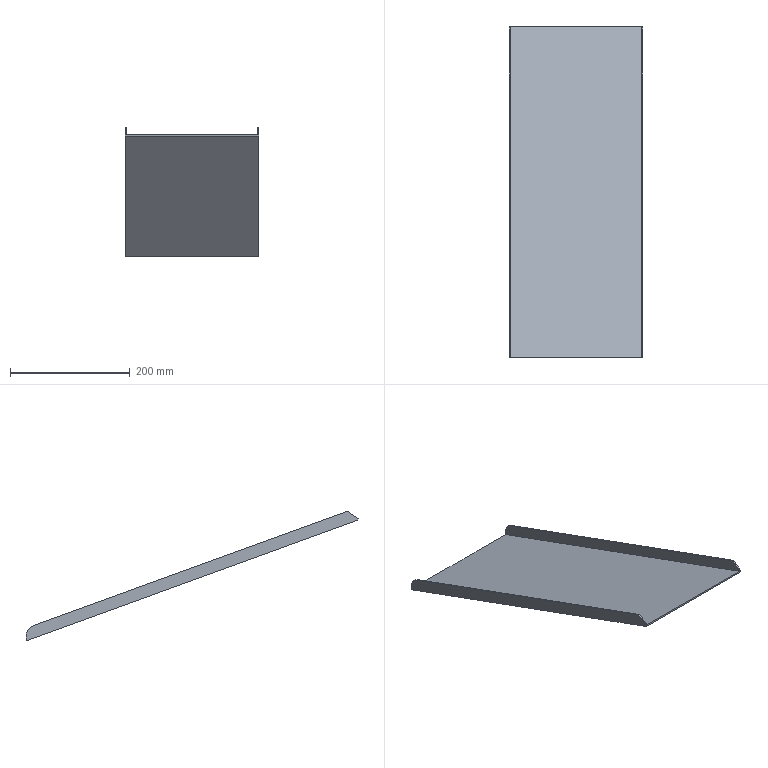Part | NX | features solid 2 | 1 solid | 14 faces | box 224.044 x 555.861 x 216.896 mm | volume 306885 mm3 | plane 9 | spline 3 | cylinder 2 | commonest cylinder face diameters 40 x2
STEP:
#1=CARTESIAN_POINT('',(-392.044,820.,-511.765));
#2=VERTEX_POINT('',#1);
#3=CARTESIAN_POINT('',(-172.,820.,-511.765));
#4=VERTEX_POINT('',#3);
#5=CARTESIAN_POINT('',(-394.044,820.,-511.765));
#6=DIRECTION('',(-1.,0.,0.));
#7=VECTOR('',#6,1000.);
#8=LINE('',#5,#7);
#9=EDGE_CURVE('',#2,#4,#8,.F.);
#10=ORIENTED_EDGE('',*,*,#9,.F.);
#11=CARTESIAN_POINT('',(-392.044,820.,-509.637));
#12=VERTEX_POINT('',#11);
#13=CARTESIAN_POINT('',(-392.044,820.,-700.));
#14=DIRECTION('',(0.,0.,-1.));
#15=VECTOR('',#14,1000.);
#16=LINE('',#13,#15);
#17=EDGE_CURVE('',#2,#12,#16,.F.);
#18=ORIENTED_EDGE('',*,*,#17,.T.);
#19=CARTESIAN_POINT('',(-172.,820.,-509.637));
#20=VERTEX_POINT('',#19);
#21=CARTESIAN_POINT('',(675.,820.,-509.637));
#22=DIRECTION('',(1.,0.,0.));
#23=VECTOR('',#22,1000.);
#24=LINE('',#21,#23);
#25=EDGE_CURVE('',#20,#12,#24,.F.);
#26=ORIENTED_EDGE('',*,*,#25,.F.);
#27=CARTESIAN_POINT('',(-172.,820.,-700.));
#28=DIRECTION('',(0.,0.,-1.));
#29=VECTOR('',#28,1000.);
#30=LINE('',#27,#29);
#31=EDGE_CURVE('',#4,#20,#30,.F.);
#32=ORIENTED_EDGE('',*,*,#31,.F.);
#33=EDGE_LOOP('',(#10,#18,#26,#32));
#34=FACE_BOUND('',#33,.T.);
#35=CARTESIAN_POINT('',(675.,820.,-700.));
#36=DIRECTION('',(0.,-1.,0.));
#37=DIRECTION('',(-1.,0.,0.));
#38=AXIS2_PLACEMENT_3D('',#35,#36,#37);
#39=PLANE('',#38);
#40=ADVANCED_FACE('',(#34),#39,.F.);
#41=CARTESIAN_POINT('',(-392.044,265.649,-307.869));
#42=VERTEX_POINT('',#41);
#43=CARTESIAN_POINT('',(-392.044,1206.032,-650.141));
#44=DIRECTION('',(0.,0.9397,-0.342));
#45=VECTOR('',#44,1000.);
#46=LINE('',#43,#45);
#47=EDGE_CURVE('',#42,#12,#46,.T.);
#48=ORIENTED_EDGE('',*,*,#47,.F.);
#49=CARTESIAN_POINT('',(-172.,265.645,-307.868));
#50=VERTEX_POINT('',#49);
#51=CARTESIAN_POINT('',(-392.044,265.649,-307.869));
#52=CARTESIAN_POINT('',(-382.876,265.644,-307.868));
#53=CARTESIAN_POINT('',(-364.539,265.649,-307.869));
#54=CARTESIAN_POINT('',(-341.617,265.581,-307.845));
#55=CARTESIAN_POINT('',(-323.28,265.66,-307.873));
#56=CARTESIAN_POINT('',(-309.528,265.272,-307.732));
#57=CARTESIAN_POINT('',(-295.775,265.417,-307.785));
#58=CARTESIAN_POINT('',(-277.438,265.558,-307.836));
#59=CARTESIAN_POINT('',(-254.517,265.652,-307.871));
#60=CARTESIAN_POINT('',(-217.843,265.608,-307.855));
#61=CARTESIAN_POINT('',(-190.337,265.641,-307.866));
#62=CARTESIAN_POINT('',(-172.,265.645,-307.868));
#63=B_SPLINE_CURVE_WITH_KNOTS('',3,(#51,#52,#53,#54,#55,#56,#57,#58,#59,#60,#61,#62),.UNSPECIFIED.,.F.,.F.,(4,1,1,1,1,1,1,1,1,4),(0.,0.02751,0.05501,0.06876,0.08252,0.09627,0.11,0.1375,0.165,0.22),.UNSPECIFIED.);
#64=EDGE_CURVE('',#42,#50,#63,.T.);
#65=ORIENTED_EDGE('',*,*,#64,.T.);
#66=CARTESIAN_POINT('',(-172.,1206.032,-650.141));
#67=DIRECTION('',(0.,0.9397,-0.342));
#68=VECTOR('',#67,1000.);
#69=LINE('',#66,#68);
#70=EDGE_CURVE('',#50,#20,#69,.T.);
#71=ORIENTED_EDGE('',*,*,#70,.T.);
#72=ORIENTED_EDGE('',*,*,#25,.T.);
#73=EDGE_LOOP('',(#48,#65,#71,#72));
#74=FACE_BOUND('',#73,.T.);
#75=CARTESIAN_POINT('',(-394.044,1206.032,-650.141));
#76=DIRECTION('',(0.,-0.342,-0.9397));
#77=DIRECTION('',(-1.,0.,0.));
#78=AXIS2_PLACEMENT_3D('',#75,#76,#77);
#79=PLANE('',#78);
#80=ADVANCED_FACE('',(#74),#79,.F.);
#81=CARTESIAN_POINT('',(-170.,808.047,-486.131));
#82=VERTEX_POINT('',#81);
#83=CARTESIAN_POINT('',(-170.,282.56,-294.869));
#84=VERTEX_POINT('',#83);
#85=CARTESIAN_POINT('',(-170.,826.84,-492.971));
#86=DIRECTION('',(0.,-0.9397,0.342));
#87=VECTOR('',#86,1000.);
#88=LINE('',#85,#87);
#89=EDGE_CURVE('',#82,#84,#88,.T.);
#90=ORIENTED_EDGE('',*,*,#89,.T.);
#91=CARTESIAN_POINT('',(-170.,265.646,-306.713));
#92=VERTEX_POINT('',#91);
#93=CARTESIAN_POINT('',(-170.,282.56,-294.869));
#94=CARTESIAN_POINT('',(-170.,276.922,-298.817));
#95=CARTESIAN_POINT('',(-170.,271.284,-302.765));
#96=CARTESIAN_POINT('',(-170.,265.646,-306.713));
#97=B_SPLINE_CURVE_WITH_KNOTS('',3,(#93,#94,#95,#96),.UNSPECIFIED.,.F.,.F.,(4,4),(0.,1.),.UNSPECIFIED.);
#98=EDGE_CURVE('',#84,#92,#97,.T.);
#99=ORIENTED_EDGE('',*,*,#98,.T.);
#100=CARTESIAN_POINT('',(-170.,265.646,-309.996));
#101=VERTEX_POINT('',#100);
#102=CARTESIAN_POINT('',(-170.,265.646,-420.));
#103=DIRECTION('',(0.,0.,-1.));
#104=VECTOR('',#103,1000.);
#105=LINE('',#102,#104);
#106=EDGE_CURVE('',#101,#92,#105,.F.);
#107=ORIENTED_EDGE('',*,*,#106,.F.);
#108=CARTESIAN_POINT('',(-170.,820.,-511.765));
#109=VERTEX_POINT('',#108);
#110=CARTESIAN_POINT('',(-170.,1205.348,-652.02));
#111=DIRECTION('',(0.,-0.9397,0.342));
#112=VECTOR('',#111,1000.);
#113=LINE('',#110,#112);
#114=EDGE_CURVE('',#109,#101,#113,.T.);
#115=ORIENTED_EDGE('',*,*,#114,.F.);
#116=CARTESIAN_POINT('',(-170.,801.206,-504.925));
#117=DIRECTION('',(-1.,0.,0.));
#118=DIRECTION('',(0.,0.,1.));
#119=AXIS2_PLACEMENT_3D('',#116,#117,#118);
#120=CIRCLE('',#119,20.);
#121=EDGE_CURVE('',#109,#82,#120,.F.);
#122=ORIENTED_EDGE('',*,*,#121,.T.);
#123=EDGE_LOOP('',(#90,#99,#107,#115,#122));
#124=FACE_BOUND('',#123,.T.);
#125=CARTESIAN_POINT('',(-170.,1206.032,-650.141));
#126=DIRECTION('',(1.,0.,0.));
#127=DIRECTION('',(0.,0.,-1.));
#128=AXIS2_PLACEMENT_3D('',#125,#126,#127);
#129=PLANE('',#128);
#130=ADVANCED_FACE('',(#124),#129,.T.);
#131=CARTESIAN_POINT('',(-394.044,265.65,-309.998));
#132=VERTEX_POINT('',#131);
#133=CARTESIAN_POINT('',(-394.044,265.65,-306.715));
#134=VERTEX_POINT('',#133);
#135=CARTESIAN_POINT('',(-394.044,265.65,-308.356));
#136=DIRECTION('',(0.,0.,-1.));
#137=VECTOR('',#136,1000.);
#138=LINE('',#135,#137);
#139=EDGE_CURVE('',#132,#134,#138,.F.);
#140=ORIENTED_EDGE('',*,*,#139,.T.);
#141=CARTESIAN_POINT('',(-394.044,282.564,-294.871));
#142=VERTEX_POINT('',#141);
#143=CARTESIAN_POINT('',(-394.044,265.65,-306.715));
#144=CARTESIAN_POINT('',(-394.044,271.288,-302.767));
#145=CARTESIAN_POINT('',(-394.044,276.926,-298.819));
#146=CARTESIAN_POINT('',(-394.044,282.564,-294.871));
#147=B_SPLINE_CURVE_WITH_KNOTS('',3,(#143,#144,#145,#146),.UNSPECIFIED.,.F.,.F.,(4,4),(0.,0.02065),.UNSPECIFIED.);
#148=EDGE_CURVE('',#134,#142,#147,.T.);
#149=ORIENTED_EDGE('',*,*,#148,.T.);
#150=CARTESIAN_POINT('',(-394.044,808.047,-486.131));
#151=VERTEX_POINT('',#150);
#152=CARTESIAN_POINT('',(-394.044,1212.188,-633.226));
#153=DIRECTION('',(0.,-0.9397,0.342));
#154=VECTOR('',#153,1000.);
#155=LINE('',#152,#154);
#156=EDGE_CURVE('',#151,#142,#155,.T.);
#157=ORIENTED_EDGE('',*,*,#156,.F.);
#158=CARTESIAN_POINT('',(-394.044,820.,-511.765));
#159=VERTEX_POINT('',#158);
#160=CARTESIAN_POINT('',(-394.044,801.206,-504.925));
#161=DIRECTION('',(-1.,0.,0.));
#162=DIRECTION('',(0.,0.,1.));
#163=AXIS2_PLACEMENT_3D('',#160,#161,#162);
#164=CIRCLE('',#163,20.);
#165=EDGE_CURVE('',#151,#159,#164,.T.);
#166=ORIENTED_EDGE('',*,*,#165,.T.);
#167=CARTESIAN_POINT('',(-394.044,1205.348,-652.02));
#168=DIRECTION('',(0.,0.9397,-0.342));
#169=VECTOR('',#168,1000.);
#170=LINE('',#167,#169);
#171=EDGE_CURVE('',#159,#132,#170,.F.);
#172=ORIENTED_EDGE('',*,*,#171,.T.);
#173=EDGE_LOOP('',(#140,#149,#157,#166,#172));
#174=FACE_BOUND('',#173,.T.);
#175=CARTESIAN_POINT('',(-394.044,1205.348,-652.02));
#176=DIRECTION('',(-1.,0.,0.));
#177=DIRECTION('',(0.,0.,1.));
#178=AXIS2_PLACEMENT_3D('',#175,#176,#177);
#179=PLANE('',#178);
#180=ADVANCED_FACE('',(#174),#179,.T.);
#181=CARTESIAN_POINT('',(-394.044,265.65,-309.998));
#182=CARTESIAN_POINT('',(-384.709,265.645,-309.996));
#183=CARTESIAN_POINT('',(-366.039,265.65,-309.998));
#184=CARTESIAN_POINT('',(-342.701,265.58,-309.973));
#185=CARTESIAN_POINT('',(-324.03,265.664,-310.003));
#186=CARTESIAN_POINT('',(-310.028,265.279,-309.863));
#187=CARTESIAN_POINT('',(-296.025,265.412,-309.911));
#188=CARTESIAN_POINT('',(-277.355,265.56,-309.966));
#189=CARTESIAN_POINT('',(-254.017,265.651,-309.999));
#190=CARTESIAN_POINT('',(-216.676,265.609,-309.983));
#191=CARTESIAN_POINT('',(-188.67,265.641,-309.995));
#192=CARTESIAN_POINT('',(-170.,265.646,-309.996));
#193=B_SPLINE_CURVE_WITH_KNOTS('',3,(#181,#182,#183,#184,#185,#186,#187,#188,#189,#190,#191,#192),.UNSPECIFIED.,.F.,.F.,(4,1,1,1,1,1,1,1,1,4),(0.003,0.03101,0.05901,0.07301,0.08702,0.101,0.115,0.143,0.171,0.227),.UNSPECIFIED.);
#194=EDGE_CURVE('',#132,#101,#193,.T.);
#195=ORIENTED_EDGE('',*,*,#194,.F.);
#196=ORIENTED_EDGE('',*,*,#171,.F.);
#197=CARTESIAN_POINT('',(-394.044,820.,-511.765));
#198=DIRECTION('',(-1.,0.,0.));
#199=VECTOR('',#198,1000.);
#200=LINE('',#197,#199);
#201=EDGE_CURVE('',#159,#2,#200,.F.);
#202=ORIENTED_EDGE('',*,*,#201,.T.);
#203=ORIENTED_EDGE('',*,*,#9,.T.);
#204=CARTESIAN_POINT('',(-170.,820.,-511.765));
#205=DIRECTION('',(1.,0.,0.));
#206=VECTOR('',#205,1000.);
#207=LINE('',#204,#206);
#208=EDGE_CURVE('',#109,#4,#207,.F.);
#209=ORIENTED_EDGE('',*,*,#208,.F.);
#210=ORIENTED_EDGE('',*,*,#114,.T.);
#211=EDGE_LOOP('',(#195,#196,#202,#203,#209,#210));
#212=FACE_BOUND('',#211,.T.);
#213=CARTESIAN_POINT('',(-394.044,1205.348,-652.02));
#214=DIRECTION('',(0.,-0.342,-0.9397));
#215=DIRECTION('',(-1.,0.,0.));
#216=AXIS2_PLACEMENT_3D('',#213,#214,#215);
#217=PLANE('',#216);
#218=ADVANCED_FACE('',(#212),#217,.T.);
#219=CARTESIAN_POINT('',(-172.,808.047,-486.131));
#220=VERTEX_POINT('',#219);
#221=CARTESIAN_POINT('',(-172.,282.56,-294.869));
#222=VERTEX_POINT('',#221);
#223=CARTESIAN_POINT('',(-172.,826.84,-492.971));
#224=DIRECTION('',(0.,-0.9397,0.342));
#225=VECTOR('',#224,1000.);
#226=LINE('',#223,#225);
#227=EDGE_CURVE('',#220,#222,#226,.T.);
#228=ORIENTED_EDGE('',*,*,#227,.T.);
#229=CARTESIAN_POINT('',(-172.,282.56,-294.869));
#230=CARTESIAN_POINT('',(-171.333,282.56,-294.869));
#231=CARTESIAN_POINT('',(-170.667,282.56,-294.869));
#232=CARTESIAN_POINT('',(-170.,282.56,-294.869));
#233=B_SPLINE_CURVE_WITH_KNOTS('',3,(#229,#230,#231,#232),.UNSPECIFIED.,.F.,.F.,(4,4),(0.,1.),.UNSPECIFIED.);
#234=EDGE_CURVE('',#222,#84,#233,.T.);
#235=ORIENTED_EDGE('',*,*,#234,.T.);
#236=ORIENTED_EDGE('',*,*,#89,.F.);
#237=CARTESIAN_POINT('',(-170.,808.047,-486.131));
#238=DIRECTION('',(-1.,0.,0.));
#239=VECTOR('',#238,1000.);
#240=LINE('',#237,#239);
#241=EDGE_CURVE('',#82,#220,#240,.T.);
#242=ORIENTED_EDGE('',*,*,#241,.T.);
#243=EDGE_LOOP('',(#228,#235,#236,#242));
#244=FACE_BOUND('',#243,.T.);
#245=CARTESIAN_POINT('',(-170.,826.84,-492.971));
#246=DIRECTION('',(0.,-0.342,-0.9397));
#247=DIRECTION('',(0.,-0.9397,0.342));
#248=AXIS2_PLACEMENT_3D('',#245,#246,#247);
#249=PLANE('',#248);
#250=ADVANCED_FACE('',(#244),#249,.F.);
#251=CARTESIAN_POINT('',(-172.,265.645,-306.713));
#252=VERTEX_POINT('',#251);
#253=CARTESIAN_POINT('',(-172.,265.645,-420.));
#254=DIRECTION('',(0.,0.,-1.));
#255=VECTOR('',#254,1000.);
#256=LINE('',#253,#255);
#257=EDGE_CURVE('',#252,#50,#256,.T.);
#258=ORIENTED_EDGE('',*,*,#257,.F.);
#259=CARTESIAN_POINT('',(-172.,265.645,-306.713));
#260=CARTESIAN_POINT('',(-172.,271.283,-302.765));
#261=CARTESIAN_POINT('',(-172.,276.921,-298.817));
#262=CARTESIAN_POINT('',(-172.,282.56,-294.869));
#263=B_SPLINE_CURVE_WITH_KNOTS('',3,(#259,#260,#261,#262),.UNSPECIFIED.,.F.,.F.,(4,4),(0.,1.),.UNSPECIFIED.);
#264=EDGE_CURVE('',#252,#222,#263,.T.);
#265=ORIENTED_EDGE('',*,*,#264,.T.);
#266=ORIENTED_EDGE('',*,*,#227,.F.);
#267=CARTESIAN_POINT('',(-172.,801.206,-504.925));
#268=DIRECTION('',(-1.,0.,0.));
#269=DIRECTION('',(0.,0.,1.));
#270=AXIS2_PLACEMENT_3D('',#267,#268,#269);
#271=CIRCLE('',#270,20.);
#272=EDGE_CURVE('',#220,#4,#271,.T.);
#273=ORIENTED_EDGE('',*,*,#272,.T.);
#274=ORIENTED_EDGE('',*,*,#31,.T.);
#275=ORIENTED_EDGE('',*,*,#70,.F.);
#276=EDGE_LOOP('',(#258,#265,#266,#273,#274,#275));
#277=FACE_BOUND('',#276,.T.);
#278=CARTESIAN_POINT('',(-172.,820.,-511.765));
#279=DIRECTION('',(-1.,0.,0.));
#280=DIRECTION('',(0.,0.,1.));
#281=AXIS2_PLACEMENT_3D('',#278,#279,#280);
#282=PLANE('',#281);
#283=ADVANCED_FACE('',(#277),#282,.T.);
#284=ORIENTED_EDGE('',*,*,#121,.F.);
#285=ORIENTED_EDGE('',*,*,#208,.T.);
#286=ORIENTED_EDGE('',*,*,#272,.F.);
#287=ORIENTED_EDGE('',*,*,#241,.F.);
#288=EDGE_LOOP('',(#284,#285,#286,#287));
#289=FACE_BOUND('',#288,.T.);
#290=CARTESIAN_POINT('',(-170.,801.206,-504.925));
#291=DIRECTION('',(-1.,0.,0.));
#292=DIRECTION('',(0.,0.,1.));
#293=AXIS2_PLACEMENT_3D('',#290,#291,#292);
#294=CYLINDRICAL_SURFACE('',#293,20.);
#295=ADVANCED_FACE('',(#289),#294,.T.);
#296=ORIENTED_EDGE('',*,*,#156,.T.);
#297=CARTESIAN_POINT('',(-392.044,282.563,-294.87));
#298=VERTEX_POINT('',#297);
#299=CARTESIAN_POINT('',(-394.044,282.564,-294.871));
#300=CARTESIAN_POINT('',(-393.378,282.564,-294.871));
#301=CARTESIAN_POINT('',(-392.711,282.564,-294.871));
#302=CARTESIAN_POINT('',(-392.044,282.563,-294.87));
#303=B_SPLINE_CURVE_WITH_KNOTS('',3,(#299,#300,#301,#302),.UNSPECIFIED.,.F.,.F.,(4,4),(0.6,1.),.UNSPECIFIED.);
#304=EDGE_CURVE('',#142,#298,#303,.T.);
#305=ORIENTED_EDGE('',*,*,#304,.T.);
#306=CARTESIAN_POINT('',(-392.044,808.047,-486.131));
#307=VERTEX_POINT('',#306);
#308=CARTESIAN_POINT('',(-392.044,826.84,-492.971));
#309=DIRECTION('',(0.,0.9397,-0.342));
#310=VECTOR('',#309,1000.);
#311=LINE('',#308,#310);
#312=EDGE_CURVE('',#307,#298,#311,.F.);
#313=ORIENTED_EDGE('',*,*,#312,.F.);
#314=CARTESIAN_POINT('',(-399.044,808.047,-486.131));
#315=DIRECTION('',(-1.,0.,0.));
#316=VECTOR('',#315,1000.);
#317=LINE('',#314,#316);
#318=EDGE_CURVE('',#307,#151,#317,.T.);
#319=ORIENTED_EDGE('',*,*,#318,.T.);
#320=EDGE_LOOP('',(#296,#305,#313,#319));
#321=FACE_BOUND('',#320,.T.);
#322=CARTESIAN_POINT('',(-399.044,826.84,-492.971));
#323=DIRECTION('',(0.,-0.342,-0.9397));
#324=DIRECTION('',(0.,-0.9397,0.342));
#325=AXIS2_PLACEMENT_3D('',#322,#323,#324);
#326=PLANE('',#325);
#327=ADVANCED_FACE('',(#321),#326,.F.);
#328=ORIENTED_EDGE('',*,*,#312,.T.);
#329=CARTESIAN_POINT('',(-392.044,265.649,-306.714));
#330=VERTEX_POINT('',#329);
#331=CARTESIAN_POINT('',(-392.044,282.563,-294.87));
#332=CARTESIAN_POINT('',(-392.044,276.925,-298.818));
#333=CARTESIAN_POINT('',(-392.044,271.287,-302.766));
#334=CARTESIAN_POINT('',(-392.044,265.649,-306.714));
#335=B_SPLINE_CURVE_WITH_KNOTS('',3,(#331,#332,#333,#334),.UNSPECIFIED.,.F.,.F.,(4,4),(0.,1.),.UNSPECIFIED.);
#336=EDGE_CURVE('',#298,#330,#335,.T.);
#337=ORIENTED_EDGE('',*,*,#336,.T.);
#338=CARTESIAN_POINT('',(-392.044,265.649,-420.));
#339=DIRECTION('',(0.,0.,-1.));
#340=VECTOR('',#339,1000.);
#341=LINE('',#338,#340);
#342=EDGE_CURVE('',#330,#42,#341,.T.);
#343=ORIENTED_EDGE('',*,*,#342,.T.);
#344=ORIENTED_EDGE('',*,*,#47,.T.);
#345=ORIENTED_EDGE('',*,*,#17,.F.);
#346=CARTESIAN_POINT('',(-392.044,801.206,-504.925));
#347=DIRECTION('',(-1.,0.,0.));
#348=DIRECTION('',(0.,0.,1.));
#349=AXIS2_PLACEMENT_3D('',#346,#347,#348);
#350=CIRCLE('',#349,20.);
#351=EDGE_CURVE('',#2,#307,#350,.F.);
#352=ORIENTED_EDGE('',*,*,#351,.T.);
#353=EDGE_LOOP('',(#328,#337,#343,#344,#345,#352));
#354=FACE_BOUND('',#353,.T.);
#355=CARTESIAN_POINT('',(-392.044,1205.348,-652.02));
#356=DIRECTION('',(-1.,0.,0.));
#357=DIRECTION('',(0.,0.,1.));
#358=AXIS2_PLACEMENT_3D('',#355,#356,#357);
#359=PLANE('',#358);
#360=ADVANCED_FACE('',(#354),#359,.F.);
#361=ORIENTED_EDGE('',*,*,#165,.F.);
#362=ORIENTED_EDGE('',*,*,#318,.F.);
#363=ORIENTED_EDGE('',*,*,#351,.F.);
#364=ORIENTED_EDGE('',*,*,#201,.F.);
#365=EDGE_LOOP('',(#361,#362,#363,#364));
#366=FACE_BOUND('',#365,.T.);
#367=CARTESIAN_POINT('',(-399.044,801.206,-504.925));
#368=DIRECTION('',(1.,0.,0.));
#369=DIRECTION('',(0.,0.,-1.));
#370=AXIS2_PLACEMENT_3D('',#367,#368,#369);
#371=CYLINDRICAL_SURFACE('',#370,20.);
#372=ADVANCED_FACE('',(#366),#371,.T.);
#373=ORIENTED_EDGE('',*,*,#342,.F.);
#374=CARTESIAN_POINT('',(-392.044,265.649,-306.714));
#375=CARTESIAN_POINT('',(-392.711,265.649,-306.714));
#376=CARTESIAN_POINT('',(-393.378,265.65,-306.714));
#377=CARTESIAN_POINT('',(-394.044,265.65,-306.715));
#378=B_SPLINE_CURVE_WITH_KNOTS('',3,(#374,#375,#376,#377),.UNSPECIFIED.,.F.,.F.,(4,4),(0.,0.4),.UNSPECIFIED.);
#379=EDGE_CURVE('',#330,#134,#378,.T.);
#380=ORIENTED_EDGE('',*,*,#379,.T.);
#381=ORIENTED_EDGE('',*,*,#139,.F.);
#382=ORIENTED_EDGE('',*,*,#194,.T.);
#383=ORIENTED_EDGE('',*,*,#106,.T.);
#384=CARTESIAN_POINT('',(-170.,265.646,-306.713));
#385=CARTESIAN_POINT('',(-170.667,265.645,-306.713));
#386=CARTESIAN_POINT('',(-171.333,265.645,-306.713));
#387=CARTESIAN_POINT('',(-172.,265.645,-306.713));
#388=B_SPLINE_CURVE_WITH_KNOTS('',3,(#384,#385,#386,#387),.UNSPECIFIED.,.F.,.F.,(4,4),(0.,1.),.UNSPECIFIED.);
#389=EDGE_CURVE('',#92,#252,#388,.T.);
#390=ORIENTED_EDGE('',*,*,#389,.T.);
#391=ORIENTED_EDGE('',*,*,#257,.T.);
#392=ORIENTED_EDGE('',*,*,#64,.F.);
#393=EDGE_LOOP('',(#373,#380,#381,#382,#383,#390,#391,#392));
#394=FACE_BOUND('',#393,.T.);
#395=CARTESIAN_POINT('',(-394.044,265.65,-306.693));
#396=CARTESIAN_POINT('',(-394.044,265.65,-310.077));
#397=CARTESIAN_POINT('',(-384.044,265.645,-306.693));
#398=CARTESIAN_POINT('',(-384.044,265.645,-310.077));
#399=CARTESIAN_POINT('',(-374.043,265.639,-306.693));
#400=CARTESIAN_POINT('',(-374.043,265.639,-310.077));
#401=CARTESIAN_POINT('',(-364.042,265.634,-306.693));
#402=CARTESIAN_POINT('',(-364.042,265.634,-310.077));
#403=CARTESIAN_POINT('',(-363.233,265.633,-306.693));
#404=CARTESIAN_POINT('',(-363.233,265.633,-310.077));
#405=CARTESIAN_POINT('',(-355.475,265.629,-306.693));
#406=CARTESIAN_POINT('',(-355.475,265.629,-310.077));
#407=CARTESIAN_POINT('',(-344.102,265.622,-306.693));
#408=CARTESIAN_POINT('',(-344.102,265.622,-310.077));
#409=CARTESIAN_POINT('',(-331.712,265.604,-306.693));
#410=CARTESIAN_POINT('',(-331.712,265.604,-310.077));
#411=CARTESIAN_POINT('',(-324.733,265.598,-306.693));
#412=CARTESIAN_POINT('',(-324.733,265.598,-310.077));
#413=CARTESIAN_POINT('',(-320.466,265.567,-306.693));
#414=CARTESIAN_POINT('',(-320.466,265.567,-310.077));
#415=CARTESIAN_POINT('',(-316.238,265.475,-306.693));
#416=CARTESIAN_POINT('',(-316.238,265.475,-310.077));
#417=CARTESIAN_POINT('',(-311.164,265.363,-306.693));
#418=CARTESIAN_POINT('',(-311.164,265.363,-310.077));
#419=CARTESIAN_POINT('',(-305.076,265.333,-306.693));
#420=CARTESIAN_POINT('',(-305.076,265.333,-310.077));
#421=CARTESIAN_POINT('',(-297.793,265.396,-306.693));
#422=CARTESIAN_POINT('',(-297.793,265.396,-310.077));
#423=CARTESIAN_POINT('',(-289.399,265.458,-306.693));
#424=CARTESIAN_POINT('',(-289.399,265.458,-310.077));
#425=CARTESIAN_POINT('',(-278.989,265.541,-306.693));
#426=CARTESIAN_POINT('',(-278.989,265.541,-310.077));
#427=CARTESIAN_POINT('',(-268.929,265.619,-306.693));
#428=CARTESIAN_POINT('',(-268.929,265.619,-310.077));
#429=CARTESIAN_POINT('',(-258.644,265.632,-306.693));
#430=CARTESIAN_POINT('',(-258.644,265.632,-310.077));
#431=CARTESIAN_POINT('',(-248.025,265.624,-306.693));
#432=CARTESIAN_POINT('',(-248.025,265.624,-310.077));
#433=CARTESIAN_POINT('',(-226.868,265.624,-306.693));
#434=CARTESIAN_POINT('',(-226.868,265.624,-310.077));
#435=CARTESIAN_POINT('',(-200.897,265.637,-306.693));
#436=CARTESIAN_POINT('',(-200.897,265.637,-310.077));
#437=CARTESIAN_POINT('',(-178.423,265.644,-306.693));
#438=CARTESIAN_POINT('',(-178.423,265.644,-310.077));
#439=CARTESIAN_POINT('',(-170.,265.646,-306.693));
#440=CARTESIAN_POINT('',(-170.,265.646,-310.077));
#441=B_SPLINE_SURFACE_WITH_KNOTS('',3,1,((#395,#396),(#397,#398),(#399,#400),(#401,#402),(#403,#404),(#405,#406),(#407,#408),(#409,#410),(#411,#412),(#413,#414),(#415,#416),(#417,#418),(#419,#420),(#421,#422),(#423,#424),(#425,#426),(#427,#428),(#429,#430),(#431,#432),(#433,#434),(#435,#436),(#437,#438),(#439,#440)),.SURF_OF_LINEAR_EXTRUSION.,.F.,.F.,.F.,(4,3,1,1,1,1,1,1,1,1,1,1,1,1,1,1,1,1,4),(2,2),(0.2365,0.2855,0.2895,0.3235,0.3405,0.349,0.3575,0.366,0.3745,0.383,0.3915,0.4085,0.4255,0.4426,0.4596,0.4766,0.4936,0.5616,0.6024),(0.3868,0.3901),.UNSPECIFIED.);
#442=ADVANCED_FACE('',(#394),#441,.F.);
#443=ORIENTED_EDGE('',*,*,#264,.F.);
#444=ORIENTED_EDGE('',*,*,#389,.F.);
#445=ORIENTED_EDGE('',*,*,#98,.F.);
#446=ORIENTED_EDGE('',*,*,#234,.F.);
#447=EDGE_LOOP('',(#443,#444,#445,#446));
#448=FACE_BOUND('',#447,.T.);
#449=CARTESIAN_POINT('',(-172.015,282.56,-294.869));
#450=CARTESIAN_POINT('',(-171.339,282.56,-294.869));
#451=CARTESIAN_POINT('',(-170.664,282.56,-294.869));
#452=CARTESIAN_POINT('',(-169.988,282.56,-294.869));
#453=CARTESIAN_POINT('',(-172.012,265.645,-306.713));
#454=CARTESIAN_POINT('',(-171.336,265.645,-306.713));
#455=CARTESIAN_POINT('',(-170.661,265.645,-306.713));
#456=CARTESIAN_POINT('',(-169.985,265.646,-306.713));
#457=B_SPLINE_SURFACE_WITH_KNOTS('',1,3,((#449,#450,#451,#452),(#453,#454,#455,#456)),.RULED_SURF.,.F.,.F.,.F.,(2,2),(4,4),(0.,1.),(0.1835,0.1856),.PIECEWISE_BEZIER_KNOTS.);
#458=ADVANCED_FACE('',(#448),#457,.T.);
#459=ORIENTED_EDGE('',*,*,#336,.F.);
#460=ORIENTED_EDGE('',*,*,#304,.F.);
#461=ORIENTED_EDGE('',*,*,#148,.F.);
#462=ORIENTED_EDGE('',*,*,#379,.F.);
#463=EDGE_LOOP('',(#459,#460,#461,#462));
#464=FACE_BOUND('',#463,.T.);
#465=CARTESIAN_POINT('',(-392.032,265.649,-306.714));
#466=CARTESIAN_POINT('',(-392.709,265.649,-306.714));
#467=CARTESIAN_POINT('',(-393.386,265.65,-306.714));
#468=CARTESIAN_POINT('',(-394.063,265.65,-306.715));
#469=CARTESIAN_POINT('',(-392.025,282.563,-294.87));
#470=CARTESIAN_POINT('',(-392.702,282.564,-294.871));
#471=CARTESIAN_POINT('',(-393.379,282.564,-294.871));
#472=CARTESIAN_POINT('',(-394.056,282.564,-294.871));
#473=B_SPLINE_SURFACE_WITH_KNOTS('',1,3,((#465,#466,#467,#468),(#469,#470,#471,#472)),.PLANE_SURF.,.F.,.F.,.F.,(2,2),(4,4),(0.,1.),(0.182,0.1841),.PIECEWISE_BEZIER_KNOTS.);
#474=ADVANCED_FACE('',(#464),#473,.T.);
#475=CLOSED_SHELL('',(#40,#80,#130,#180,#218,#250,#283,#295,#327,#360,#372,#442,#458,#474));
#476=MANIFOLD_SOLID_BREP('',#475);
#477=(LENGTH_UNIT()NAMED_UNIT(*)SI_UNIT(.MILLI.,.METRE.));
#478=UNCERTAINTY_MEASURE_WITH_UNIT(LENGTH_MEASURE(0.1016),#477,'','');
#479=(NAMED_UNIT(*)PLANE_ANGLE_UNIT()SI_UNIT($,.RADIAN.));
#480=(NAMED_UNIT(*)SI_UNIT($,.STERADIAN.)SOLID_ANGLE_UNIT());
#481=(GEOMETRIC_REPRESENTATION_CONTEXT(3)GLOBAL_UNCERTAINTY_ASSIGNED_CONTEXT((#478))GLOBAL_UNIT_ASSIGNED_CONTEXT((#477,#479,#480))REPRESENTATION_CONTEXT('',''));
#482=ADVANCED_BREP_SHAPE_REPRESENTATION('',(#476),#481);